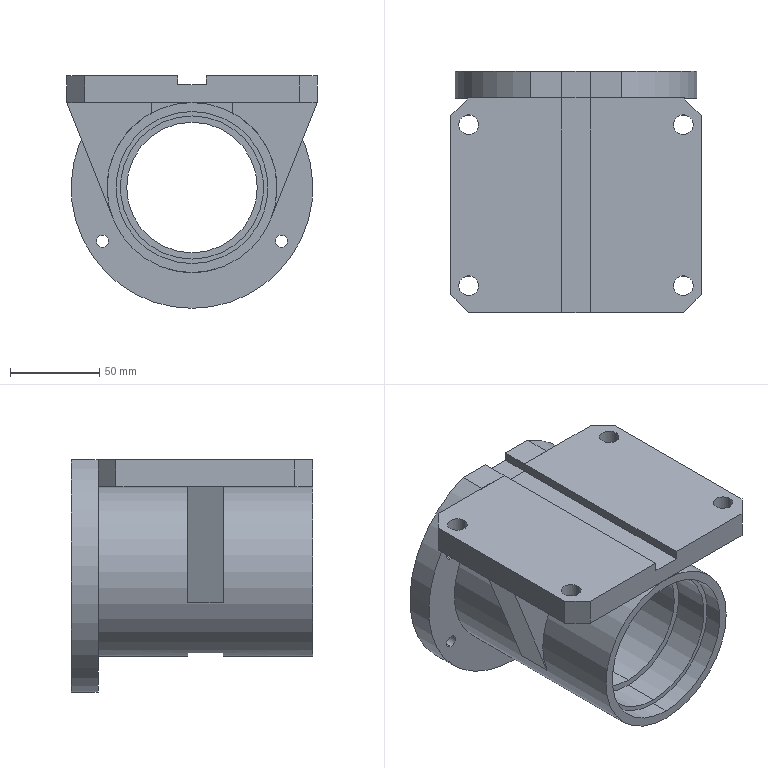Part | STEP file | YCD14007A-08.03.07.04 Bearing Seat | 5 solids | 78 faces | box 140 x 135 x 130 mm | volume 675590 mm3 | plane 42 | cylinder 36 | commonest cylinder face diameters 6.8 x8 11 x8 85 x6 80 x4 95 x4 7 x2